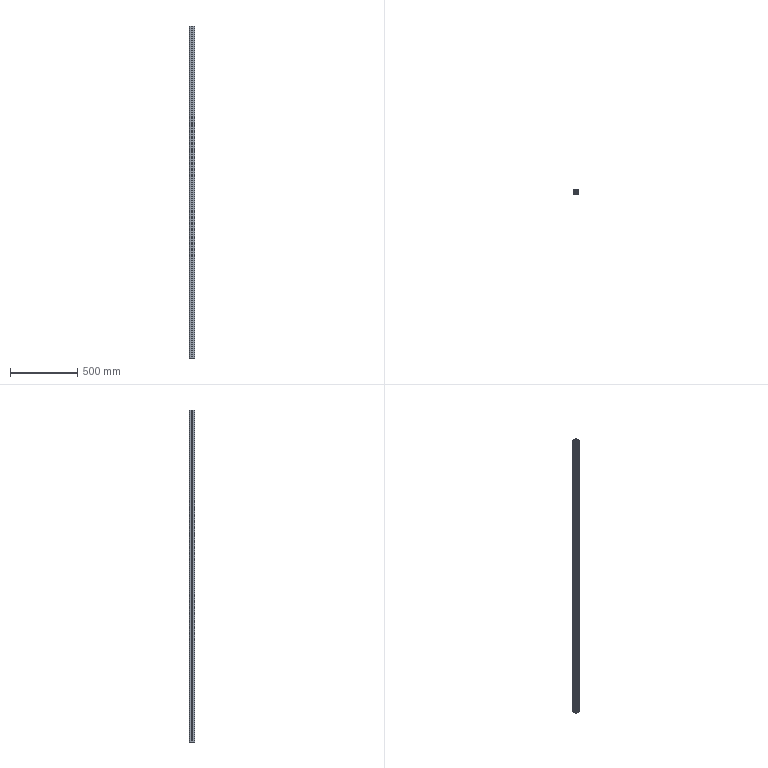Part | SolidWorks | features HoleWzd 2, Extrusion 1 | 1 solid | 244 faces | box 40 x 40 x 2470 mm | volume 1483507 mm3 | plane 171 | cylinder 73 | commonest cylinder face diameters 6.6 x21 6.8 x15 11 x12 1 x8 2 x8 5 x4